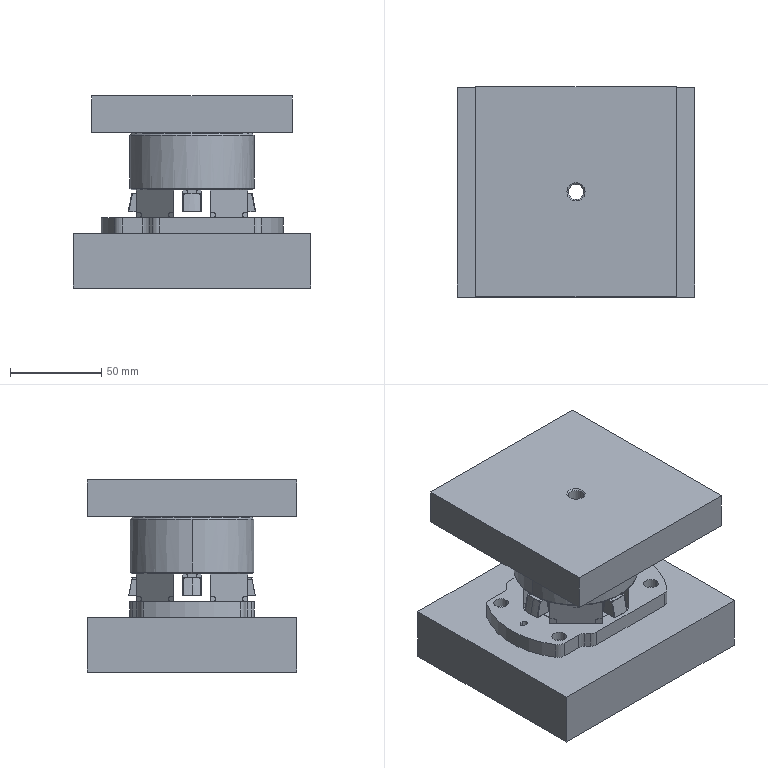NC program | NX | posted with a generic post | part box 130 x 115 x 105.2 mm
Lines 1409 to 2217 of 4507:
(PLANAR_MILL_1_1 , TOOL : ER25-D2.5-23)
N2738 T14 M6
N2740 G54
N2742 G17 G0 G90 X-6.853 Y-7.999 S6500 M3
N2744 G43 Z94. H14
N2746 G94 G1 Z35.141 F4500.
N2748 X-6.601 Y-8.133 Z35.126 F1000.
N2750 X-6.268 Y-8.148 Z35.109
N2752 X-5.96 Y-8.02 Z35.091
N2754 X-5.737 Y-7.772 Z35.074
N2756 X-5.653 Y-7.541 Z35.061
N2758 X-5.665 Y-7.207 Z35.043
N2760 X-5.818 Y-6.911 Z35.026
N2762 X-6.083 Y-6.709 Z35.008
N2764 X-6.41 Y-6.64 Z34.991
N2766 X-6.652 Y-6.683 Z34.978
N2768 X-6.889 Y-6.818 Z34.964
N2770 X-7.063 Y-7.028 Z34.949
N2772 X-7.147 Y-7.259 Z34.936
N2774 X-7.148 Y-7.532 Z34.922
N2776 X-7.053 Y-7.788 Z34.908
N2778 X-6.895 Y-7.977 Z34.895
N2780 X-6.601 Y-8.133 Z34.877
N2782 X-6.268 Y-8.148 Z34.86
N2784 X-5.96 Y-8.02 Z34.843
N2786 X-5.737 Y-7.772 Z34.825
N2788 X-5.653 Y-7.541 Z34.812
N2790 X-5.665 Y-7.207 Z34.795
N2792 X-5.818 Y-6.911 Z34.777
N2794 X-6.083 Y-6.709 Z34.76
N2796 X-6.41 Y-6.64 Z34.742
N2798 X-6.652 Y-6.683 Z34.729
N2800 X-6.889 Y-6.818 Z34.715
N2802 X-7.063 Y-7.028 Z34.701
N2804 X-7.147 Y-7.259 Z34.688
N2806 X-7.148 Y-7.532 Z34.674
N2808 X-7.053 Y-7.788 Z34.659
N2810 X-6.895 Y-7.977 Z34.646
N2812 X-6.601 Y-8.133 Z34.629
N2814 X-6.268 Y-8.148 Z34.611
N2816 X-5.96 Y-8.02 Z34.594
N2818 X-5.737 Y-7.772 Z34.576
N2820 X-5.653 Y-7.541 Z34.564
N2822 X-5.665 Y-7.207 Z34.546
N2824 X-5.818 Y-6.911 Z34.529
N2826 X-6.083 Y-6.709 Z34.511
N2828 X-6.41 Y-6.64 Z34.494
N2830 X-6.652 Y-6.683 Z34.481
N2832 X-6.889 Y-6.818 Z34.467
N2834 X-7.063 Y-7.028 Z34.452
N2836 X-7.147 Y-7.259 Z34.439
N2838 X-7.148 Y-7.532 Z34.425
N2840 X-7.053 Y-7.788 Z34.411
N2842 X-6.895 Y-7.977 Z34.398
N2844 X-6.601 Y-8.133 Z34.38
N2846 X-6.268 Y-8.148 Z34.363
N2848 X-5.96 Y-8.02 Z34.345
N2850 X-5.737 Y-7.772 Z34.328
N2852 X-5.653 Y-7.541 Z34.315
N2854 X-5.665 Y-7.207 Z34.298
N2856 X-5.818 Y-6.911 Z34.28
N2858 X-6.083 Y-6.709 Z34.263
N2860 X-6.41 Y-6.64 Z34.245
N2862 X-6.652 Y-6.683 Z34.232
N2864 X-6.889 Y-6.818 Z34.218
N2866 X-7.063 Y-7.028 Z34.204
N2868 X-7.147 Y-7.259 Z34.191
N2870 X-7.148 Y-7.532 Z34.176
N2872 X-7.053 Y-7.788 Z34.162
N2874 X-6.895 Y-7.977 Z34.149
N2876 X-6.601 Y-8.133 Z34.132
N2878 X-6.268 Y-8.148 Z34.114
N2880 X-5.96 Y-8.02 Z34.097
N2882 X-5.737 Y-7.772 Z34.079
N2884 X-5.653 Y-7.541 Z34.066
N2886 X-5.665 Y-7.207 Z34.049
N2888 X-5.818 Y-6.911 Z34.032
N2890 X-6.083 Y-6.709 Z34.014
N2892 X-6.41 Y-6.64 Z33.997
N2894 X-6.652 Y-6.683 Z33.984
N2896 X-6.889 Y-6.818 Z33.969
N2898 X-7.063 Y-7.028 Z33.955
N2900 X-7.147 Y-7.259 Z33.942
N2902 X-7.148 Y-7.532 Z33.928
N2904 X-7.053 Y-7.788 Z33.914
N2906 X-6.895 Y-7.977 Z33.901
N2908 X-6.601 Y-8.133 Z33.883
N2910 X-6.268 Y-8.148 Z33.866
N2912 X-5.96 Y-8.02 Z33.848
N2914 X-5.737 Y-7.772 Z33.831
N2916 X-5.653 Y-7.541 Z33.818
N2918 X-5.665 Y-7.207 Z33.8
N2920 X-5.818 Y-6.911 Z33.783
N2922 X-6.083 Y-6.709 Z33.765
N2924 X-6.41 Y-6.64 Z33.748
N2926 X-6.652 Y-6.683 Z33.735
N2928 X-6.889 Y-6.818 Z33.721
N2930 X-7.063 Y-7.028 Z33.706
N2932 X-7.147 Y-7.259 Z33.694
N2934 X-7.148 Y-7.532 Z33.679
N2936 X-7.053 Y-7.788 Z33.665
N2938 X-6.895 Y-7.977 Z33.652
N2940 X-6.601 Y-8.133 Z33.635
N2942 X-6.268 Y-8.148 Z33.617
N2944 X-5.96 Y-8.02 Z33.6
N2946 X-5.737 Y-7.772 Z33.582
N2948 X-5.653 Y-7.541 Z33.569
N2950 X-5.665 Y-7.207 Z33.552
N2952 X-5.818 Y-6.911 Z33.534
N2954 X-6.083 Y-6.709 Z33.517
N2956 X-6.41 Y-6.64 Z33.499
N2958 X-6.652 Y-6.683 Z33.487
N2960 X-6.889 Y-6.818 Z33.472
N2962 X-7.063 Y-7.028 Z33.458
N2964 X-7.147 Y-7.259 Z33.445
N2966 X-7.148 Y-7.532 Z33.431
N2968 X-7.053 Y-7.788 Z33.416
N2970 X-6.895 Y-7.977 Z33.404
N2972 X-6.601 Y-8.133 Z33.386
N2974 X-6.268 Y-8.148 Z33.369
N2976 X-5.96 Y-8.02 Z33.351
N2978 X-5.737 Y-7.772 Z33.334
N2980 X-5.653 Y-7.541 Z33.321
N2982 X-5.665 Y-7.207 Z33.303
N2984 X-5.818 Y-6.911 Z33.286
N2986 X-6.083 Y-6.709 Z33.268
N2988 X-6.41 Y-6.64 Z33.251
N2990 X-6.652 Y-6.683 Z33.238
N2992 X-6.889 Y-6.818 Z33.224
N2994 X-7.063 Y-7.028 Z33.209
N2996 X-7.147 Y-7.259 Z33.196
N2998 X-7.148 Y-7.532 Z33.182
N3000 X-7.053 Y-7.788 Z33.168
N3002 X-6.895 Y-7.977 Z33.155
N3004 X-6.601 Y-8.133 Z33.137
N3006 X-6.268 Y-8.148 Z33.12
N3008 X-5.96 Y-8.02 Z33.103
N3010 X-5.737 Y-7.772 Z33.085
N3012 X-5.653 Y-7.541 Z33.072
N3014 X-5.665 Y-7.207 Z33.055
N3016 X-5.818 Y-6.911 Z33.037
N3018 X-6.083 Y-6.709 Z33.02
N3020 X-6.41 Y-6.64 Z33.002
N3022 X-6.652 Y-6.683 Z32.989
N3024 X-6.889 Y-6.818 Z32.975
N3026 X-7.063 Y-7.028 Z32.961
N3028 X-7.147 Y-7.259 Z32.948
N3030 X-7.148 Y-7.532 Z32.934
N3032 X-7.053 Y-7.788 Z32.919
N3034 X-6.895 Y-7.977 Z32.906
N3036 X-6.601 Y-8.133 Z32.889
N3038 X-6.268 Y-8.148 Z32.871
N3040 X-5.96 Y-8.02 Z32.854
N3042 X-5.737 Y-7.772 Z32.836
N3044 X-5.653 Y-7.541 Z32.824
N3046 X-5.665 Y-7.207 Z32.806
N3048 X-5.818 Y-6.911 Z32.789
N3050 X-6.083 Y-6.709 Z32.771
N3052 X-6.41 Y-6.64 Z32.754
N3054 X-6.652 Y-6.683 Z32.741
N3056 X-6.889 Y-6.818 Z32.726
N3058 X-7.063 Y-7.028 Z32.712
N3060 X-7.147 Y-7.259 Z32.699
N3062 X-7.148 Y-7.532 Z32.685
N3064 X-7.053 Y-7.788 Z32.671
N3066 X-6.895 Y-7.977 Z32.658
N3068 X-6.601 Y-8.133 Z32.64
N3070 X-6.268 Y-8.148 Z32.623
N3072 X-5.96 Y-8.02 Z32.605
N3074 X-5.737 Y-7.772 Z32.588
N3076 X-5.653 Y-7.541 Z32.575
N3078 X-5.665 Y-7.207 Z32.558
N3080 X-5.818 Y-6.911 Z32.54
N3082 X-6.083 Y-6.709 Z32.523
N3084 X-6.41 Y-6.64 Z32.505
N3086 X-6.652 Y-6.683 Z32.492
N3088 X-6.889 Y-6.818 Z32.478
N3090 X-7.063 Y-7.028 Z32.464
N3092 X-7.147 Y-7.259 Z32.451
N3094 X-7.148 Y-7.532 Z32.436
N3096 X-7.053 Y-7.788 Z32.422
N3098 X-6.895 Y-7.977 Z32.409
N3100 X-6.601 Y-8.133 Z32.392
N3102 X-6.268 Y-8.148 Z32.374
N3104 X-5.96 Y-8.02 Z32.357
N3106 X-5.737 Y-7.772 Z32.339
N3108 X-5.653 Y-7.541 Z32.326
N3110 X-5.665 Y-7.207 Z32.309
N3112 X-5.818 Y-6.911 Z32.291
N3114 X-6.083 Y-6.709 Z32.274
N3116 X-6.41 Y-6.64 Z32.257
N3118 X-6.652 Y-6.683 Z32.244
N3120 X-6.889 Y-6.818 Z32.229
N3122 X-7.063 Y-7.028 Z32.215
N3124 X-7.147 Y-7.259 Z32.202
N3126 X-7.148 Y-7.532 Z32.188
N3128 X-7.053 Y-7.788 Z32.174
N3130 X-6.895 Y-7.977 Z32.161
N3132 X-6.601 Y-8.133 Z32.143
N3134 X-6.268 Y-8.148 Z32.126
N3136 X-5.96 Y-8.02 Z32.108
N3138 X-5.737 Y-7.772 Z32.091
N3140 X-5.653 Y-7.541 Z32.078
N3142 X-5.665 Y-7.207 Z32.06
N3144 X-5.818 Y-6.911 Z32.043
N3146 X-6.083 Y-6.709 Z32.025
N3148 X-6.41 Y-6.64 Z32.008
N3150 X-6.652 Y-6.683 Z31.995
N3152 X-6.889 Y-6.818 Z31.981
N3154 X-7.063 Y-7.028 Z31.966
N3156 X-7.147 Y-7.259 Z31.954
N3158 X-7.148 Y-7.532 Z31.939
N3160 X-7.053 Y-7.788 Z31.925
N3162 X-6.895 Y-7.977 Z31.912
N3164 X-6.601 Y-8.133 Z31.895
N3166 X-6.268 Y-8.148 Z31.877
N3168 X-5.96 Y-8.02 Z31.86
N3170 X-5.737 Y-7.772 Z31.842
N3172 X-5.653 Y-7.541 Z31.829
N3174 X-5.665 Y-7.207 Z31.812
N3176 X-5.818 Y-6.911 Z31.794
N3178 X-6.083 Y-6.709 Z31.777
N3180 X-6.41 Y-6.64 Z31.759
N3182 X-6.652 Y-6.683 Z31.747
N3184 X-6.889 Y-6.818 Z31.732
N3186 X-7.063 Y-7.028 Z31.718
N3188 X-7.147 Y-7.259 Z31.705
N3190 X-7.148 Y-7.532 Z31.691
N3192 X-7.053 Y-7.788 Z31.676
N3194 X-6.895 Y-7.977 Z31.664
N3196 X-6.601 Y-8.133 Z31.646
N3198 X-6.268 Y-8.148 Z31.629
N3200 X-5.96 Y-8.02 Z31.611
N3202 X-5.737 Y-7.772 Z31.594
N3204 X-5.653 Y-7.541 Z31.581
N3206 X-5.665 Y-7.207 Z31.563
N3208 X-5.818 Y-6.911 Z31.546
N3210 X-6.083 Y-6.709 Z31.528
N3212 X-6.41 Y-6.64 Z31.511
N3214 X-6.652 Y-6.683 Z31.498
N3216 X-6.889 Y-6.818 Z31.484
N3218 X-7.063 Y-7.028 Z31.469
N3220 X-7.147 Y-7.259 Z31.456
N3222 X-7.148 Y-7.532 Z31.442
N3224 X-7.053 Y-7.788 Z31.428
N3226 X-6.895 Y-7.977 Z31.415
N3228 X-6.601 Y-8.133 Z31.397
N3230 X-6.268 Y-8.148 Z31.38
N3232 X-5.96 Y-8.02 Z31.363
N3234 X-5.737 Y-7.772 Z31.345
N3236 X-5.653 Y-7.541 Z31.332
N3238 X-5.665 Y-7.207 Z31.315
N3240 X-5.818 Y-6.911 Z31.297
N3242 X-6.083 Y-6.709 Z31.28
N3244 X-6.41 Y-6.64 Z31.262
N3246 X-6.652 Y-6.683 Z31.249
N3248 X-6.889 Y-6.818 Z31.235
N3250 X-7.063 Y-7.028 Z31.221
N3252 X-7.147 Y-7.259 Z31.208
N3254 X-7.148 Y-7.532 Z31.194
N3256 X-7.053 Y-7.788 Z31.179
N3258 X-6.895 Y-7.977 Z31.166
N3260 X-6.601 Y-8.133 Z31.149
N3262 X-6.268 Y-8.148 Z31.131
N3264 X-5.96 Y-8.02 Z31.114
N3266 X-5.737 Y-7.772 Z31.096
N3268 X-5.653 Y-7.541 Z31.084
N3270 X-5.665 Y-7.207 Z31.066
N3272 X-5.818 Y-6.911 Z31.049
N3274 X-6.083 Y-6.709 Z31.031
N3276 X-6.41 Y-6.64 Z31.014
N3278 X-6.652 Y-6.683 Z31.001
N3280 X-6.889 Y-6.818 Z30.986
N3282 X-7.063 Y-7.028 Z30.972
N3284 X-7.147 Y-7.259 Z30.959
N3286 X-7.148 Y-7.532 Z30.945
N3288 X-7.053 Y-7.788 Z30.931
N3290 X-6.895 Y-7.977 Z30.918
N3292 X-6.601 Y-8.133 Z30.9
N3294 X-6.268 Y-8.148 Z30.883
N3296 X-5.96 Y-8.02 Z30.865
N3298 X-5.737 Y-7.772 Z30.848
N3300 X-5.653 Y-7.541 Z30.835
N3302 X-5.665 Y-7.207 Z30.818
N3304 X-5.818 Y-6.911 Z30.8
N3306 X-6.083 Y-6.709 Z30.783
N3308 X-6.41 Y-6.64 Z30.765
N3310 X-6.652 Y-6.683 Z30.752
N3312 X-6.889 Y-6.818 Z30.738
N3314 X-7.063 Y-7.028 Z30.724
N3316 X-7.147 Y-7.259 Z30.711
N3318 X-7.148 Y-7.532 Z30.696
N3320 X-7.053 Y-7.788 Z30.682
N3322 X-6.895 Y-7.977 Z30.669
N3324 X-6.601 Y-8.133 Z30.652
N3326 X-6.268 Y-8.148 Z30.634
N3328 X-5.96 Y-8.02 Z30.617
N3330 X-5.737 Y-7.772 Z30.599
N3332 X-5.653 Y-7.541 Z30.586
N3334 X-5.665 Y-7.207 Z30.569
N3336 X-5.818 Y-6.911 Z30.551
N3338 X-6.083 Y-6.709 Z30.534
N3340 X-6.41 Y-6.64 Z30.517
N3342 X-6.652 Y-6.683 Z30.504
N3344 X-6.889 Y-6.818 Z30.489
N3346 X-7.063 Y-7.028 Z30.475
N3348 X-7.147 Y-7.259 Z30.462
N3350 X-7.148 Y-7.532 Z30.448
N3352 X-7.053 Y-7.788 Z30.434
N3354 X-6.895 Y-7.977 Z30.421
N3356 X-6.601 Y-8.133 Z30.403
N3358 X-6.268 Y-8.148 Z30.386
N3360 X-5.96 Y-8.02 Z30.368
N3362 X-5.737 Y-7.772 Z30.351
N3364 X-5.653 Y-7.541 Z30.338
N3366 X-5.665 Y-7.207 Z30.32
N3368 X-5.818 Y-6.911 Z30.303
N3370 X-6.083 Y-6.709 Z30.285
N3372 X-6.41 Y-6.64 Z30.268
N3374 X-6.652 Y-6.683 Z30.255
N3376 X-6.889 Y-6.818 Z30.241
N3378 X-7.063 Y-7.028 Z30.226
N3380 X-7.147 Y-7.259 Z30.214
N3382 X-7.148 Y-7.532 Z30.199
N3384 X-7.053 Y-7.788 Z30.185
N3386 X-6.895 Y-7.977 Z30.172
N3388 X-6.601 Y-8.133 Z30.155
N3390 X-6.268 Y-8.148 Z30.137
N3392 X-5.96 Y-8.02 Z30.12
N3394 X-5.737 Y-7.772 Z30.102
N3396 X-5.653 Y-7.541 Z30.089
N3398 X-5.665 Y-7.207 Z30.072
N3400 X-5.818 Y-6.911 Z30.054
N3402 X-6.083 Y-6.709 Z30.037
N3404 X-6.41 Y-6.64 Z30.019
N3406 X-6.652 Y-6.683 Z30.007
N3408 X-6.889 Y-6.818 Z29.992
N3410 X-7.063 Y-7.028 Z29.978
N3412 X-7.147 Y-7.259 Z29.965
N3414 X-7.148 Y-7.532 Z29.951
N3416 X-7.053 Y-7.788 Z29.936
N3418 X-6.895 Y-7.977 Z29.924
N3420 X-6.601 Y-8.133 Z29.906
N3422 X-6.268 Y-8.148 Z29.889
N3424 X-5.96 Y-8.02 Z29.871
N3426 X-5.737 Y-7.772 Z29.854
N3428 X-5.653 Y-7.541 Z29.841
N3430 X-5.665 Y-7.207 Z29.823
N3432 X-5.818 Y-6.911 Z29.806
N3434 X-6.083 Y-6.709 Z29.788
N3436 X-6.41 Y-6.64 Z29.771
N3438 X-6.652 Y-6.683 Z29.758
N3440 X-6.889 Y-6.818 Z29.744
N3442 X-7.063 Y-7.028 Z29.729
N3444 X-7.147 Y-7.259 Z29.716
N3446 X-7.148 Y-7.532 Z29.702
N3448 X-7.053 Y-7.788 Z29.688
N3450 X-6.895 Y-7.977 Z29.675
N3452 X-6.601 Y-8.133 Z29.657
N3454 X-6.268 Y-8.148 Z29.64
N3456 X-5.96 Y-8.02 Z29.623
N3458 X-5.737 Y-7.772 Z29.605
N3460 X-5.653 Y-7.541 Z29.592
N3462 X-5.665 Y-7.207 Z29.575
N3464 X-5.818 Y-6.911 Z29.557
N3466 X-6.083 Y-6.709 Z29.54
N3468 X-6.41 Y-6.64 Z29.522
N3470 X-6.652 Y-6.683 Z29.509
N3472 X-6.889 Y-6.818 Z29.495
N3474 X-7.063 Y-7.028 Z29.481
N3476 X-7.147 Y-7.259 Z29.468
N3478 X-7.148 Y-7.532 Z29.454
N3480 X-7.053 Y-7.788 Z29.439
N3482 X-6.895 Y-7.977 Z29.426
N3484 X-6.601 Y-8.133 Z29.409
N3486 X-6.268 Y-8.148 Z29.391
N3488 X-5.96 Y-8.02 Z29.374
N3490 X-5.737 Y-7.772 Z29.356
N3492 X-5.653 Y-7.541 Z29.344
N3494 X-5.665 Y-7.207 Z29.326
N3496 X-5.818 Y-6.911 Z29.309
N3498 X-6.083 Y-6.709 Z29.291
N3500 X-6.41 Y-6.64 Z29.274
N3502 X-6.652 Y-6.683 Z29.261
N3504 X-6.889 Y-6.818 Z29.246
N3506 X-7.063 Y-7.028 Z29.232
N3508 X-7.147 Y-7.259 Z29.219
N3510 X-7.148 Y-7.532 Z29.205
N3512 X-7.053 Y-7.788 Z29.191
N3514 X-6.895 Y-7.977 Z29.178
N3516 X-6.601 Y-8.133 Z29.16
N3518 X-6.268 Y-8.148 Z29.143
N3520 X-5.96 Y-8.02 Z29.125
N3522 X-5.737 Y-7.772 Z29.108
N3524 X-5.653 Y-7.541 Z29.095
N3526 X-5.665 Y-7.207 Z29.078
N3528 X-5.818 Y-6.911 Z29.06
N3530 X-6.083 Y-6.709 Z29.043
N3532 X-6.41 Y-6.64 Z29.025
N3534 X-6.652 Y-6.683 Z29.012
N3536 X-6.889 Y-6.818 Z28.998
N3538 X-7.063 Y-7.028 Z28.984
N3540 X-7.147 Y-7.259 Z28.971
N3542 X-7.148 Y-7.532 Z28.956
N3544 X-7.053 Y-7.788 Z28.942
N3546 X-6.895 Y-7.977 Z28.929
N3548 X-6.601 Y-8.133 Z28.912
N3550 X-6.268 Y-8.148 Z28.894
N3552 X-5.96 Y-8.02 Z28.877
N3554 X-5.737 Y-7.772 Z28.859
N3556 X-5.653 Y-7.541 Z28.846
N3558 X-5.665 Y-7.207 Z28.829
N3560 X-5.818 Y-6.911 Z28.811
N3562 X-6.083 Y-6.709 Z28.794
N3564 X-6.41 Y-6.64 Z28.777
N3566 X-6.652 Y-6.683 Z28.764
N3568 X-6.889 Y-6.818 Z28.749
N3570 X-7.063 Y-7.028 Z28.735
N3572 X-7.147 Y-7.259 Z28.722
N3574 X-7.148 Y-7.532 Z28.708
N3576 X-7.053 Y-7.788 Z28.694
N3578 X-6.895 Y-7.977 Z28.681
N3580 X-6.601 Y-8.133 Z28.663
N3582 X-6.268 Y-8.148 Z28.646
N3584 X-5.96 Y-8.02 Z28.628
N3586 X-5.737 Y-7.772 Z28.611
N3588 X-5.653 Y-7.541 Z28.598
N3590 X-5.665 Y-7.207 Z28.58
N3592 X-5.818 Y-6.911 Z28.563
N3594 X-6.083 Y-6.709 Z28.545
N3596 X-6.41 Y-6.64 Z28.528
N3598 X-6.652 Y-6.683 Z28.515
N3600 X-6.889 Y-6.818 Z28.501
N3602 X-7.063 Y-7.028 Z28.486
N3604 X-7.147 Y-7.259 Z28.474
N3606 X-7.148 Y-7.532 Z28.459
N3608 X-7.053 Y-7.788 Z28.445
N3610 X-6.895 Y-7.977 Z28.432
N3612 X-6.601 Y-8.133 Z28.415
N3614 X-6.268 Y-8.148 Z28.397
N3616 X-5.96 Y-8.02 Z28.38
N3618 X-5.737 Y-7.772 Z28.362
N3620 X-5.653 Y-7.541 Z28.349
N3622 X-5.665 Y-7.207 Z28.332
N3624 X-5.818 Y-6.911 Z28.314
N3626 X-6.083 Y-6.709 Z28.297
N3628 X-6.41 Y-6.64 Z28.279
N3630 X-6.652 Y-6.683 Z28.267
N3632 X-6.889 Y-6.818 Z28.252
N3634 X-7.063 Y-7.028 Z28.238
N3636 X-7.147 Y-7.259 Z28.225
N3638 X-7.148 Y-7.532 Z28.211
N3640 X-7.053 Y-7.788 Z28.196
N3642 X-6.895 Y-7.977 Z28.184
N3644 X-6.601 Y-8.133 Z28.166
N3646 X-6.268 Y-8.148 Z28.149
N3648 X-5.96 Y-8.02 Z28.131
N3650 X-5.737 Y-7.772 Z28.114
N3652 X-5.653 Y-7.541 Z28.101
N3654 X-5.665 Y-7.207 Z28.083
N3656 X-5.818 Y-6.911 Z28.066
N3658 X-6.083 Y-6.709 Z28.048
N3660 X-6.41 Y-6.64 Z28.031
N3662 X-6.652 Y-6.683 Z28.018
N3664 X-6.889 Y-6.818 Z28.004
N3666 X-7.063 Y-7.028 Z27.989
N3668 X-7.147 Y-7.259 Z27.976
N3670 X-7.148 Y-7.532 Z27.962
N3672 X-7.053 Y-7.788 Z27.948
N3674 X-6.895 Y-7.977 Z27.935
N3676 X-6.601 Y-8.133 Z27.917
N3678 X-6.268 Y-8.148 Z27.9
N3680 X-5.96 Y-8.02 Z27.883
N3682 X-5.737 Y-7.772 Z27.865
N3684 X-5.653 Y-7.541 Z27.852
N3686 X-5.665 Y-7.207 Z27.835
N3688 X-5.818 Y-6.911 Z27.817
N3690 X-6.083 Y-6.709 Z27.8
N3692 X-6.41 Y-6.64 Z27.782
N3694 X-6.652 Y-6.683 Z27.769
N3696 X-6.889 Y-6.818 Z27.755
N3698 X-7.063 Y-7.028 Z27.741
N3700 X-7.147 Y-7.259 Z27.728
N3702 X-7.148 Y-7.532 Z27.714
N3704 X-7.053 Y-7.788 Z27.699
N3706 X-6.895 Y-7.977 Z27.686
N3708 X-6.601 Y-8.133 Z27.669
N3710 X-6.268 Y-8.148 Z27.651
N3712 X-5.96 Y-8.02 Z27.634
N3714 X-5.737 Y-7.772 Z27.616
N3716 X-5.653 Y-7.541 Z27.604
N3718 X-5.665 Y-7.207 Z27.586
N3720 X-5.818 Y-6.911 Z27.569
N3722 X-6.083 Y-6.709 Z27.551
N3724 X-6.41 Y-6.64 Z27.534
N3726 X-6.652 Y-6.683 Z27.521
N3728 X-6.889 Y-6.818 Z27.506
N3730 X-7.063 Y-7.028 Z27.492
N3732 X-7.147 Y-7.259 Z27.479
N3734 X-7.148 Y-7.532 Z27.465
N3736 X-7.053 Y-7.788 Z27.451
N3738 X-6.895 Y-7.977 Z27.438
N3740 X-6.601 Y-8.133 Z27.42
N3742 X-6.268 Y-8.148 Z27.403
N3744 X-5.96 Y-8.02 Z27.385
N3746 X-5.737 Y-7.772 Z27.368
N3748 X-5.653 Y-7.541 Z27.355
N3750 X-5.665 Y-7.207 Z27.338
N3752 X-5.818 Y-6.911 Z27.32
N3754 X-6.083 Y-6.709 Z27.303
N3756 X-6.41 Y-6.64 Z27.285
N3758 X-6.652 Y-6.683 Z27.272
N3760 X-6.889 Y-6.818 Z27.258
N3762 X-7.063 Y-7.028 Z27.244
N3764 X-7.147 Y-7.259 Z27.231
N3766 X-7.148 Y-7.532 Z27.216
N3768 X-7.053 Y-7.788 Z27.202
N3770 X-6.895 Y-7.977 Z27.189
N3772 X-6.601 Y-8.133 Z27.172
N3774 X-6.268 Y-8.148 Z27.154
N3776 X-5.96 Y-8.02 Z27.137
N3778 X-5.737 Y-7.772 Z27.119
N3780 X-5.653 Y-7.541 Z27.106
N3782 X-5.665 Y-7.207 Z27.089
N3784 X-5.818 Y-6.911 Z27.071
N3786 X-6.083 Y-6.709 Z27.054
N3788 X-6.41 Y-6.64 Z27.037
N3790 X-6.652 Y-6.683 Z27.024
N3792 X-6.889 Y-6.818 Z27.009
N3794 X-7.063 Y-7.028 Z26.995
N3796 X-7.147 Y-7.259 Z26.982
N3798 X-7.148 Y-7.532 Z26.968
N3800 X-7.053 Y-7.788 Z26.954
N3802 X-6.895 Y-7.977 Z26.941
N3804 X-6.601 Y-8.133 Z26.923
N3806 X-6.268 Y-8.148 Z26.906
N3808 X-5.96 Y-8.02 Z26.888
N3810 X-5.737 Y-7.772 Z26.871
N3812 X-5.653 Y-7.541 Z26.858
N3814 X-5.665 Y-7.207 Z26.84
N3816 X-5.818 Y-6.911 Z26.823
N3818 X-6.083 Y-6.709 Z26.805
N3820 X-6.41 Y-6.64 Z26.788
N3822 X-6.652 Y-6.683 Z26.775
N3824 X-6.889 Y-6.818 Z26.761
N3826 X-7.063 Y-7.028 Z26.746
N3828 X-7.147 Y-7.259 Z26.734
N3830 X-7.148 Y-7.532 Z26.719
N3832 X-7.053 Y-7.788 Z26.705
N3834 X-6.895 Y-7.977 Z26.692
N3836 X-6.601 Y-8.133 Z26.675
N3838 X-6.268 Y-8.148 Z26.657
N3840 X-5.96 Y-8.02 Z26.64
N3842 X-5.737 Y-7.772 Z26.622
N3844 X-5.653 Y-7.541 Z26.609
N3846 X-5.665 Y-7.207 Z26.592
N3848 X-5.818 Y-6.911 Z26.574
N3850 X-6.083 Y-6.709 Z26.557
N3852 X-6.41 Y-6.64 Z26.539
N3854 X-6.652 Y-6.683 Z26.526
N3856 X-6.889 Y-6.818 Z26.512
N3858 X-7.063 Y-7.028 Z26.498
N3860 X-7.147 Y-7.259 Z26.485
N3862 X-7.148 Y-7.532 Z26.471
N3864 X-7.053 Y-7.788 Z26.456
N3866 X-6.895 Y-7.977 Z26.443
N3868 X-6.601 Y-8.133 Z26.426
N3870 X-6.268 Y-8.148 Z26.409
N3872 X-5.96 Y-8.02 Z26.391
N3874 X-5.737 Y-7.772 Z26.374
N3876 X-5.653 Y-7.541 Z26.361
N3878 X-5.665 Y-7.207 Z26.343
N3880 X-5.818 Y-6.911 Z26.326
N3882 X-6.083 Y-6.709 Z26.308
N3884 X-6.41 Y-6.64 Z26.291
N3886 X-6.652 Y-6.683 Z26.278
N3888 X-6.889 Y-6.818 Z26.264
N3890 X-7.063 Y-7.028 Z26.249
N3892 X-7.147 Y-7.259 Z26.236
N3894 X-7.148 Y-7.532 Z26.222
N3896 X-7.053 Y-7.788 Z26.208
N3898 X-6.895 Y-7.977 Z26.195
N3900 X-6.601 Y-8.133 Z26.177
N3902 X-6.268 Y-8.148 Z26.16
N3904 X-5.96 Y-8.02 Z26.142
N3906 X-5.737 Y-7.772 Z26.125
N3908 X-5.653 Y-7.541 Z26.112
N3910 X-5.665 Y-7.207 Z26.095
N3912 X-5.818 Y-6.911 Z26.077
N3914 X-6.083 Y-6.709 Z26.06
N3916 X-6.41 Y-6.64 Z26.042
N3918 X-6.652 Y-6.683 Z26.029
N3920 X-6.889 Y-6.818 Z26.015
N3922 X-7.063 Y-7.028 Z26.001
N3924 X-7.147 Y-7.259 Z25.988
N3926 X-7.148 Y-7.532 Z25.974
N3928 X-7.053 Y-7.788 Z25.959
N3930 X-6.895 Y-7.977 Z25.946
N3932 X-6.601 Y-8.133 Z25.929
N3934 X-6.268 Y-8.148 Z25.911
N3936 X-5.96 Y-8.02 Z25.894
N3938 X-5.737 Y-7.772 Z25.876
N3940 X-5.653 Y-7.541 Z25.864
N3942 X-5.665 Y-7.207 Z25.846
N3944 X-5.818 Y-6.911 Z25.829
N3946 X-6.083 Y-6.709 Z25.811
N3948 X-6.41 Y-6.64 Z25.794
N3950 X-6.652 Y-6.683 Z25.781
N3952 X-6.889 Y-6.818 Z25.766
N3954 X-7.063 Y-7.028 Z25.752
N3956 X-7.147 Y-7.259 Z25.739
N3958 X-7.148 Y-7.532 Z25.725
N3960 X-7.053 Y-7.788 Z25.711
N3962 X-6.895 Y-7.977 Z25.698
N3964 X-6.601 Y-8.133 Z25.68
N3966 X-6.268 Y-8.148 Z25.663
N3968 X-5.96 Y-8.02 Z25.645
N3970 X-5.737 Y-7.772 Z25.628
N3972 X-5.653 Y-7.541 Z25.615
N3974 X-5.665 Y-7.207 Z25.598
N3976 X-5.818 Y-6.911 Z25.58
N3978 X-6.083 Y-6.709 Z25.563
N3980 X-6.41 Y-6.64 Z25.545
N3982 X-6.652 Y-6.683 Z25.532
N3984 X-6.889 Y-6.818 Z25.518
N3986 X-7.063 Y-7.028 Z25.504
N3988 X-7.147 Y-7.259 Z25.491
N3990 X-7.148 Y-7.532 Z25.476
N3992 X-7.053 Y-7.788 Z25.462
N3994 X-6.895 Y-7.977 Z25.449
N3996 X-6.601 Y-8.133 Z25.432
N3998 X-6.268 Y-8.148 Z25.414
N4000 X-5.96 Y-8.02 Z25.397
N4002 X-5.737 Y-7.772 Z25.379
N4004 X-5.653 Y-7.541 Z25.366
N4006 X-5.665 Y-7.207 Z25.349
N4008 X-5.818 Y-6.911 Z25.331
N4010 X-6.083 Y-6.709 Z25.314
N4012 X-6.41 Y-6.64 Z25.297
N4014 X-6.652 Y-6.683 Z25.284
N4016 X-6.889 Y-6.818 Z25.269
N4018 X-7.063 Y-7.028 Z25.255
N4020 X-7.147 Y-7.259 Z25.242
N4022 X-7.148 Y-7.532 Z25.228
N4024 X-7.053 Y-7.788 Z25.214
N4026 X-6.895 Y-7.977 Z25.201
N4028 X-6.601 Y-8.133 Z25.183
N4030 X-6.268 Y-8.148 Z25.166
N4032 X-5.96 Y-8.02 Z25.148
N4034 X-5.737 Y-7.772 Z25.131
N4036 X-5.653 Y-7.541 Z25.118
N4038 X-5.665 Y-7.207 Z25.1
N4040 X-5.818 Y-6.911 Z25.083
N4042 X-6.083 Y-6.709 Z25.065
N4044 X-6.41 Y-6.64 Z25.048
N4046 X-6.652 Y-6.683 Z25.035
N4048 X-6.889 Y-6.818 Z25.021
N4050 X-7.063 Y-7.028 Z25.006
N4052 X-7.105 Y-7.144 Z25.
N4054 G3 X-6.656 Y-8.105 R0.75
N4056 X-7.105 Y-7.144 R-0.75
N4058 X-7.112 Y-7.635 R0.75
N4060 X-6.165 Y-8.112 R0.75
N4062 G1 Z25.5
N4064 G0 Z94.
(PLANAR_MILL_1_1_COPY , TOOL : ER25-D2.5-23)
N4066 G18 X-6.853 Z-7.999
N4068 Y-94.
N4070 G1 Y-35.141 F4500.
N4072 X-6.601 Y-35.126 Z-8.133 F1000.
N4074 X-6.268 Y-35.109 Z-8.148
N4076 X-5.96 Y-35.091 Z-8.02
N4078 X-5.737 Y-35.074 Z-7.772
N4080 X-5.653 Y-35.061 Z-7.541
N4082 X-5.665 Y-35.043 Z-7.207
N4084 X-5.818 Y-35.026 Z-6.911
N4086 X-6.083 Y-35.008 Z-6.709
N4088 X-6.41 Y-34.991 Z-6.64
N4090 X-6.652 Y-34.978 Z-6.683
N4092 X-6.889 Y-34.964 Z-6.818
N4094 X-7.063 Y-34.949 Z-7.028
N4096 X-7.147 Y-34.936 Z-7.259
N4098 X-7.148 Y-34.922 Z-7.532
N4100 X-7.053 Y-34.908 Z-7.788
N4102 X-6.895 Y-34.895 Z-7.977
N4104 X-6.601 Y-34.877 Z-8.133
N4106 X-6.268 Y-34.86 Z-8.148
N4108 X-5.96 Y-34.843 Z-8.02
N4110 X-5.737 Y-34.825 Z-7.772
N4112 X-5.653 Y-34.812 Z-7.541
N4114 X-5.665 Y-34.795 Z-7.207
N4116 X-5.818 Y-34.777 Z-6.911
N4118 X-6.083 Y-34.76 Z-6.709
N4120 X-6.41 Y-34.742 Z-6.64
N4122 X-6.652 Y-34.729 Z-6.683
N4124 X-6.889 Y-34.715 Z-6.818
N4126 X-7.063 Y-34.701 Z-7.028
N4128 X-7.147 Y-34.688 Z-7.259
N4130 X-7.148 Y-34.674 Z-7.532
N4132 X-7.053 Y-34.659 Z-7.788
N4134 X-6.895 Y-34.646 Z-7.977
N4136 X-6.601 Y-34.629 Z-8.133
N4138 X-6.268 Y-34.611 Z-8.148
N4140 X-5.96 Y-34.594 Z-8.02
N4142 X-5.737 Y-34.576 Z-7.772
N4144 X-5.653 Y-34.564 Z-7.541
N4146 X-5.665 Y-34.546 Z-7.207
N4148 X-5.818 Y-34.529 Z-6.911
N4150 X-6.083 Y-34.511 Z-6.709
N4152 X-6.41 Y-34.494 Z-6.64
N4154 X-6.652 Y-34.481 Z-6.683
N4156 X-6.889 Y-34.467 Z-6.818
N4158 X-7.063 Y-34.452 Z-7.028
N4160 X-7.147 Y-34.439 Z-7.259
N4162 X-7.148 Y-34.425 Z-7.532
N4164 X-7.053 Y-34.411 Z-7.788
N4166 X-6.895 Y-34.398 Z-7.977
N4168 X-6.601 Y-34.38 Z-8.133
N4170 X-6.268 Y-34.363 Z-8.148
N4172 X-5.96 Y-34.345 Z-8.02
N4174 X-5.737 Y-34.328 Z-7.772
N4176 X-5.653 Y-34.315 Z-7.541
N4178 X-5.665 Y-34.298 Z-7.207
N4180 X-5.818 Y-34.28 Z-6.911
N4182 X-6.083 Y-34.263 Z-6.709
N4184 X-6.41 Y-34.245 Z-6.64
N4186 X-6.652 Y-34.232 Z-6.683
N4188 X-6.889 Y-34.218 Z-6.818
N4190 X-7.063 Y-34.204 Z-7.028
N4192 X-7.147 Y-34.191 Z-7.259
N4194 X-7.148 Y-34.176 Z-7.532
N4196 X-7.053 Y-34.162 Z-7.788
N4198 X-6.895 Y-34.149 Z-7.977
N4200 X-6.601 Y-34.132 Z-8.133
N4202 X-6.268 Y-34.114 Z-8.148
N4204 X-5.96 Y-34.097 Z-8.02
N4206 X-5.737 Y-34.079 Z-7.772
N4208 X-5.653 Y-34.066 Z-7.541
N4210 X-5.665 Y-34.049 Z-7.207
N4212 X-5.818 Y-34.032 Z-6.911
N4214 X-6.083 Y-34.014 Z-6.709
N4216 X-6.41 Y-33.997 Z-6.64
N4218 X-6.652 Y-33.984 Z-6.683
N4220 X-6.889 Y-33.969 Z-6.818
N4222 X-7.063 Y-33.955 Z-7.028
N4224 X-7.147 Y-33.942 Z-7.259
N4226 X-7.148 Y-33.928 Z-7.532
N4228 X-7.053 Y-33.914 Z-7.788
N4230 X-6.895 Y-33.901 Z-7.977
N4232 X-6.601 Y-33.883 Z-8.133
N4234 X-6.268 Y-33.866 Z-8.148
N4236 X-5.96 Y-33.848 Z-8.02
N4238 X-5.737 Y-33.831 Z-7.772
N4240 X-5.653 Y-33.818 Z-7.541
N4242 X-5.665 Y-33.8 Z-7.207
N4244 X-5.818 Y-33.783 Z-6.911
N4246 X-6.083 Y-33.765 Z-6.709
N4248 X-6.41 Y-33.748 Z-6.64
N4250 X-6.652 Y-33.735 Z-6.683
N4252 X-6.889 Y-33.721 Z-6.818
N4254 X-7.063 Y-33.706 Z-7.028
N4256 X-7.147 Y-33.694 Z-7.259
N4258 X-7.148 Y-33.679 Z-7.532
N4260 X-7.053 Y-33.665 Z-7.788
N4262 X-6.895 Y-33.652 Z-7.977
N4264 X-6.601 Y-33.635 Z-8.133
N4266 X-6.268 Y-33.617 Z-8.148
N4268 X-5.96 Y-33.6 Z-8.02
N4270 X-5.737 Y-33.582 Z-7.772
N4272 X-5.653 Y-33.569 Z-7.541
N4274 X-5.665 Y-33.552 Z-7.207
N4276 X-5.818 Y-33.534 Z-6.911
N4278 X-6.083 Y-33.517 Z-6.709
N4280 X-6.41 Y-33.499 Z-6.64
N4282 X-6.652 Y-33.487 Z-6.683
N4284 X-6.889 Y-33.472 Z-6.818
N4286 X-7.063 Y-33.458 Z-7.028
N4288 X-7.147 Y-33.445 Z-7.259
N4290 X-7.148 Y-33.431 Z-7.532
N4292 X-7.053 Y-33.416 Z-7.788
N4294 X-6.895 Y-33.404 Z-7.977
N4296 X-6.601 Y-33.386 Z-8.133
N4298 X-6.268 Y-33.369 Z-8.148
N4300 X-5.96 Y-33.351 Z-8.02
N4302 X-5.737 Y-33.334 Z-7.772
N4304 X-5.653 Y-33.321 Z-7.541
N4306 X-5.665 Y-33.303 Z-7.207
N4308 X-5.818 Y-33.286 Z-6.911
N4310 X-6.083 Y-33.268 Z-6.709
N4312 X-6.41 Y-33.251 Z-6.64
N4314 X-6.652 Y-33.238 Z-6.683
N4316 X-6.889 Y-33.224 Z-6.818
N4318 X-7.063 Y-33.209 Z-7.028
N4320 X-7.147 Y-33.196 Z-7.259
N4322 X-7.148 Y-33.182 Z-7.532
N4324 X-7.053 Y-33.168 Z-7.788
N4326 X-6.895 Y-33.155 Z-7.977
N4328 X-6.601 Y-33.137 Z-8.133
N4330 X-6.268 Y-33.12 Z-8.148
N4332 X-5.96 Y-33.103 Z-8.02
N4334 X-5.737 Y-33.085 Z-7.772
N4336 X-5.653 Y-33.072 Z-7.541
N4338 X-5.665 Y-33.055 Z-7.207
N4340 X-5.818 Y-33.037 Z-6.911
N4342 X-6.083 Y-33.02 Z-6.709